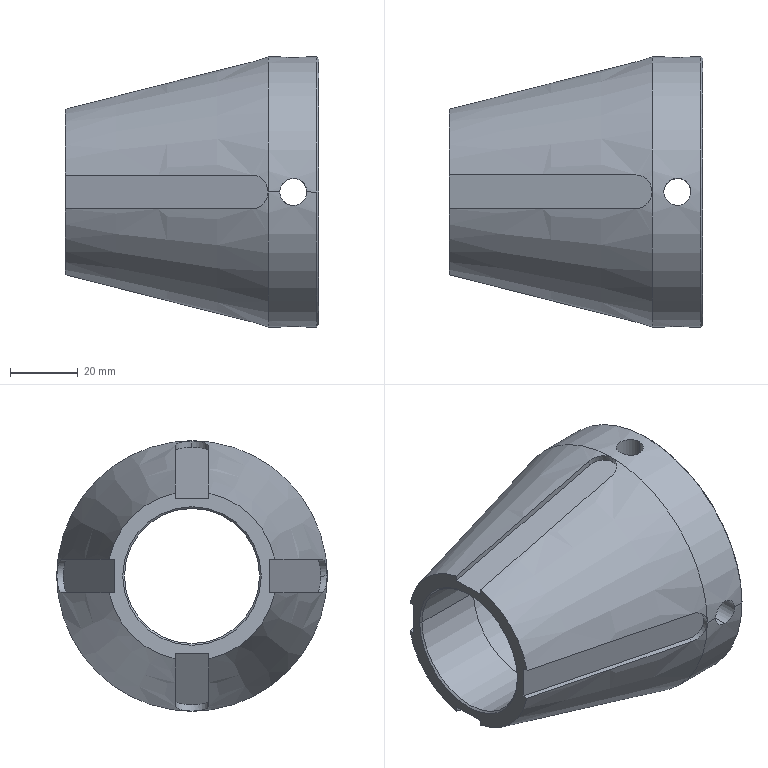Part | STEP file | Coil positioning piece 1 | 1 solid | 46 faces | box 75 x 80 x 80 mm | volume 140418 mm3 | cylinder 20 | plane 14 | cone 12 | commonest cylinder face diameters 8 x8 10 x6 40 x2 49.835 x2 80 x2